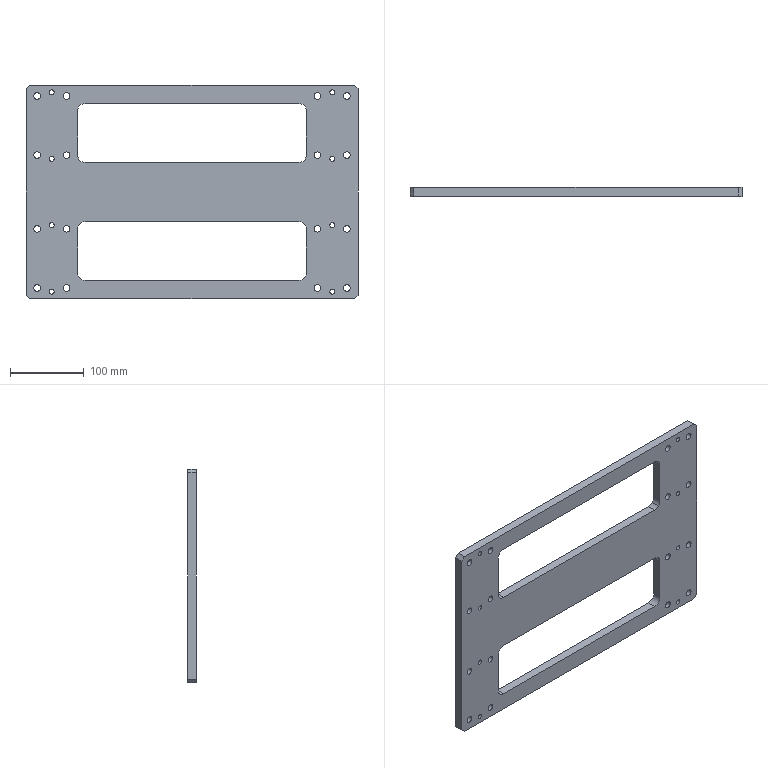Part | STEP file | CENTERING.MOUNT.stp | 1 solid | 102 faces | box 450 x 12 x 290 mm | volume 953602 mm3 | spline 47 | cylinder 40 | plane 15 | commonest cylinder face diameters 9 x16 6.6 x8 11 x8 20 x8